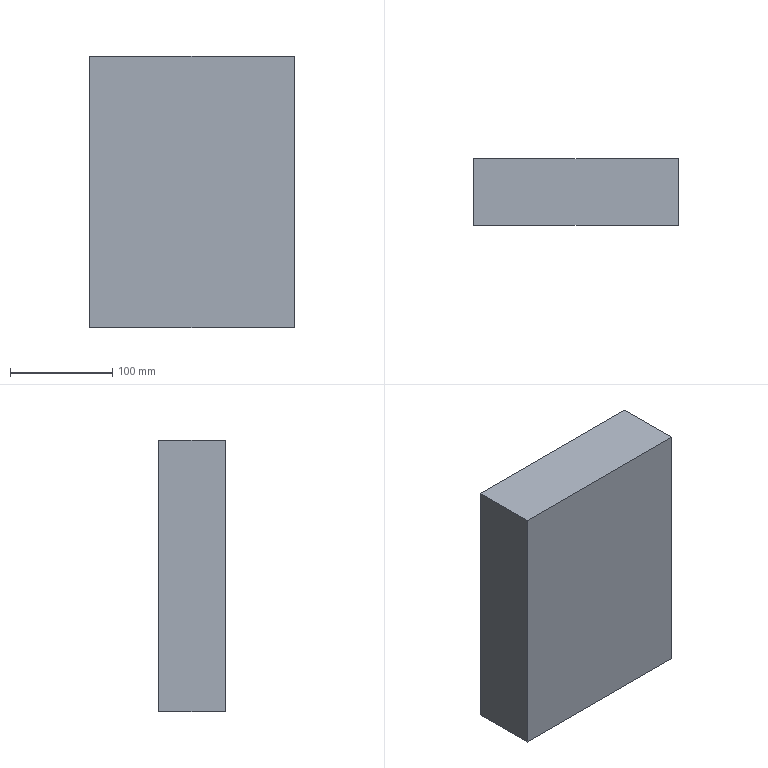Part | STEP file | lll_id3718_x_t | 1 solid | 10 faces | box 200 x 65 x 265 mm | volume 3423738 mm3 | plane 6 | cylinder 2 | cone 2 | commonest cylinder face diameters 17.505 x2
STEP:
#1=CARTESIAN_POINT('',(1843.188,637.5,-370.));
#2=VERTEX_POINT('',#1);
#3=CARTESIAN_POINT('',(1834.435,637.5,-370.));
#4=DIRECTION('',(0.,0.,1.));
#5=DIRECTION('',(1.,0.,0.));
#6=AXIS2_PLACEMENT_3D('',#3,#4,#5);
#7=CIRCLE('',#6,8.752);
#8=EDGE_CURVE('',#2,#2,#7,.T.);
#9=ORIENTED_EDGE('',*,*,#8,.T.);
#10=EDGE_LOOP('',(#9));
#11=FACE_BOUND('',#10,.T.);
#12=CARTESIAN_POINT('',(1809.435,670.,-370.));
#13=VERTEX_POINT('',#12);
#14=CARTESIAN_POINT('',(2009.435,670.,-370.));
#15=VERTEX_POINT('',#14);
#16=CARTESIAN_POINT('',(4038.751,670.,-370.));
#17=DIRECTION('',(1.,0.,0.));
#18=VECTOR('',#17,1.);
#19=LINE('',#16,#18);
#20=EDGE_CURVE('',#13,#15,#19,.T.);
#21=ORIENTED_EDGE('',*,*,#20,.T.);
#22=CARTESIAN_POINT('',(2009.435,605.,-370.));
#23=VERTEX_POINT('',#22);
#24=CARTESIAN_POINT('',(2009.435,1.,-370.));
#25=DIRECTION('',(0.,1.,0.));
#26=VECTOR('',#25,1.);
#27=LINE('',#24,#26);
#28=EDGE_CURVE('',#23,#15,#27,.T.);
#29=ORIENTED_EDGE('',*,*,#28,.F.);
#30=CARTESIAN_POINT('',(1809.435,605.,-370.));
#31=VERTEX_POINT('',#30);
#32=CARTESIAN_POINT('',(4038.751,605.,-370.));
#33=DIRECTION('',(1.,0.,0.));
#34=VECTOR('',#33,1.);
#35=LINE('',#32,#34);
#36=EDGE_CURVE('',#31,#23,#35,.T.);
#37=ORIENTED_EDGE('',*,*,#36,.F.);
#38=CARTESIAN_POINT('',(1809.435,636.5,-370.));
#39=DIRECTION('',(0.,-1.,0.));
#40=VECTOR('',#39,1.);
#41=LINE('',#38,#40);
#42=EDGE_CURVE('',#13,#31,#41,.T.);
#43=ORIENTED_EDGE('',*,*,#42,.F.);
#44=EDGE_LOOP('',(#21,#29,#37,#43));
#45=FACE_BOUND('',#44,.T.);
#46=CARTESIAN_POINT('',(1993.188,637.5,-370.));
#47=VERTEX_POINT('',#46);
#48=CARTESIAN_POINT('',(1984.435,637.5,-370.));
#49=DIRECTION('',(0.,0.,1.));
#50=DIRECTION('',(1.,0.,0.));
#51=AXIS2_PLACEMENT_3D('',#48,#49,#50);
#52=CIRCLE('',#51,8.752);
#53=EDGE_CURVE('',#47,#47,#52,.T.);
#54=ORIENTED_EDGE('',*,*,#53,.T.);
#55=EDGE_LOOP('',(#54));
#56=FACE_BOUND('',#55,.T.);
#57=CARTESIAN_POINT('',(4038.751,1.,-370.));
#58=DIRECTION('',(0.,0.,-1.));
#59=DIRECTION('',(-1.,0.,0.));
#60=AXIS2_PLACEMENT_3D('',#57,#58,#59);
#61=PLANE('',#60);
#62=ADVANCED_FACE('',(#11,#45,#56),#61,.T.);
#63=CARTESIAN_POINT('',(2009.435,605.,-105.));
#64=VERTEX_POINT('',#63);
#65=CARTESIAN_POINT('',(2009.435,605.,-180.));
#66=DIRECTION('',(0.,0.,-1.));
#67=VECTOR('',#66,1.);
#68=LINE('',#65,#67);
#69=EDGE_CURVE('',#64,#23,#68,.T.);
#70=ORIENTED_EDGE('',*,*,#69,.F.);
#71=CARTESIAN_POINT('',(1809.435,605.,-105.));
#72=VERTEX_POINT('',#71);
#73=CARTESIAN_POINT('',(2154.435,605.,-105.));
#74=DIRECTION('',(1.,0.,0.));
#75=VECTOR('',#74,1.);
#76=LINE('',#73,#75);
#77=EDGE_CURVE('',#72,#64,#76,.T.);
#78=ORIENTED_EDGE('',*,*,#77,.F.);
#79=CARTESIAN_POINT('',(1809.435,605.,-180.));
#80=DIRECTION('',(0.,0.,-1.));
#81=VECTOR('',#80,1.);
#82=LINE('',#79,#81);
#83=EDGE_CURVE('',#72,#31,#82,.T.);
#84=ORIENTED_EDGE('',*,*,#83,.T.);
#85=ORIENTED_EDGE('',*,*,#36,.T.);
#86=EDGE_LOOP('',(#70,#78,#84,#85));
#87=FACE_OUTER_BOUND('',#86,.T.);
#88=CARTESIAN_POINT('',(2052.435,605.,-180.));
#89=DIRECTION('',(0.,1.,0.));
#90=DIRECTION('',(1.,0.,0.));
#91=AXIS2_PLACEMENT_3D('',#88,#89,#90);
#92=PLANE('',#91);
#93=ADVANCED_FACE('',(#87),#92,.F.);
#94=ORIENTED_EDGE('',*,*,#83,.F.);
#95=CARTESIAN_POINT('',(1809.435,670.,-105.));
#96=VERTEX_POINT('',#95);
#97=CARTESIAN_POINT('',(1809.435,593.,-105.));
#98=DIRECTION('',(0.,-1.,0.000000092));
#99=VECTOR('',#98,1.);
#100=LINE('',#97,#99);
#101=EDGE_CURVE('',#96,#72,#100,.T.);
#102=ORIENTED_EDGE('',*,*,#101,.F.);
#103=CARTESIAN_POINT('',(1809.435,670.,-180.));
#104=DIRECTION('',(0.,0.,-1.));
#105=VECTOR('',#104,1.);
#106=LINE('',#103,#105);
#107=EDGE_CURVE('',#96,#13,#106,.T.);
#108=ORIENTED_EDGE('',*,*,#107,.T.);
#109=ORIENTED_EDGE('',*,*,#42,.T.);
#110=EDGE_LOOP('',(#94,#102,#108,#109));
#111=FACE_OUTER_BOUND('',#110,.T.);
#112=CARTESIAN_POINT('',(1809.435,636.5,-180.));
#113=DIRECTION('',(1.,0.,0.));
#114=DIRECTION('',(0.,-1.,0.));
#115=AXIS2_PLACEMENT_3D('',#112,#113,#114);
#116=PLANE('',#115);
#117=ADVANCED_FACE('',(#111),#116,.F.);
#118=ORIENTED_EDGE('',*,*,#107,.F.);
#119=CARTESIAN_POINT('',(2009.435,670.,-105.));
#120=VERTEX_POINT('',#119);
#121=CARTESIAN_POINT('',(2154.435,670.,-105.));
#122=DIRECTION('',(1.,0.,0.));
#123=VECTOR('',#122,1.);
#124=LINE('',#121,#123);
#125=EDGE_CURVE('',#96,#120,#124,.T.);
#126=ORIENTED_EDGE('',*,*,#125,.T.);
#127=CARTESIAN_POINT('',(2009.435,670.,-180.));
#128=DIRECTION('',(0.,0.,-1.));
#129=VECTOR('',#128,1.);
#130=LINE('',#127,#129);
#131=EDGE_CURVE('',#120,#15,#130,.T.);
#132=ORIENTED_EDGE('',*,*,#131,.T.);
#133=ORIENTED_EDGE('',*,*,#20,.F.);
#134=EDGE_LOOP('',(#118,#126,#132,#133));
#135=FACE_OUTER_BOUND('',#134,.T.);
#136=CARTESIAN_POINT('',(1983.435,670.,-180.));
#137=DIRECTION('',(0.,1.,0.));
#138=DIRECTION('',(1.,0.,0.));
#139=AXIS2_PLACEMENT_3D('',#136,#137,#138);
#140=PLANE('',#139);
#141=ADVANCED_FACE('',(#135),#140,.T.);
#142=CARTESIAN_POINT('',(2009.435,600.,-105.));
#143=DIRECTION('',(0.,1.,-0.000000092));
#144=VECTOR('',#143,1.);
#145=LINE('',#142,#144);
#146=EDGE_CURVE('',#64,#120,#145,.T.);
#147=ORIENTED_EDGE('',*,*,#146,.F.);
#148=ORIENTED_EDGE('',*,*,#69,.T.);
#149=ORIENTED_EDGE('',*,*,#28,.T.);
#150=ORIENTED_EDGE('',*,*,#131,.F.);
#151=EDGE_LOOP('',(#147,#148,#149,#150));
#152=FACE_OUTER_BOUND('',#151,.T.);
#153=CARTESIAN_POINT('',(2009.435,600.,-180.));
#154=DIRECTION('',(1.,0.,0.));
#155=DIRECTION('',(0.,0.,1.));
#156=AXIS2_PLACEMENT_3D('',#153,#154,#155);
#157=PLANE('',#156);
#158=ADVANCED_FACE('',(#152),#157,.T.);
#159=ORIENTED_EDGE('',*,*,#125,.F.);
#160=ORIENTED_EDGE('',*,*,#101,.T.);
#161=ORIENTED_EDGE('',*,*,#77,.T.);
#162=ORIENTED_EDGE('',*,*,#146,.T.);
#163=EDGE_LOOP('',(#159,#160,#161,#162));
#164=FACE_OUTER_BOUND('',#163,.T.);
#165=CARTESIAN_POINT('',(2154.435,593.,-105.));
#166=DIRECTION('',(0.,-0.000000092,-1.));
#167=DIRECTION('',(-1.,0.,0.));
#168=AXIS2_PLACEMENT_3D('',#165,#166,#167);
#169=PLANE('',#168);
#170=ADVANCED_FACE('',(#164),#169,.F.);
#171=CARTESIAN_POINT('',(1843.188,637.5,-328.747));
#172=VERTEX_POINT('',#171);
#173=CARTESIAN_POINT('',(1834.435,637.5,-328.747));
#174=DIRECTION('',(0.,0.,1.));
#175=DIRECTION('',(1.,0.,0.));
#176=AXIS2_PLACEMENT_3D('',#173,#174,#175);
#177=CIRCLE('',#176,8.752);
#178=EDGE_CURVE('',#172,#172,#177,.T.);
#179=ORIENTED_EDGE('',*,*,#178,.T.);
#180=EDGE_LOOP('',(#179));
#181=FACE_BOUND('',#180,.T.);
#182=ORIENTED_EDGE('',*,*,#8,.F.);
#183=EDGE_LOOP('',(#182));
#184=FACE_BOUND('',#183,.T.);
#185=CARTESIAN_POINT('',(1834.435,637.5,-370.));
#186=DIRECTION('',(0.,0.,1.));
#187=DIRECTION('',(-1.,0.,0.));
#188=AXIS2_PLACEMENT_3D('',#185,#186,#187);
#189=CYLINDRICAL_SURFACE('',#188,8.752);
#190=ADVANCED_FACE('',(#181,#184),#189,.F.);
#191=CARTESIAN_POINT('',(1834.435,637.5,-319.994));
#192=VERTEX_POINT('',#191);
#193=VERTEX_LOOP('',#192);
#194=FACE_BOUND('',#193,.T.);
#195=ORIENTED_EDGE('',*,*,#178,.F.);
#196=EDGE_LOOP('',(#195));
#197=FACE_BOUND('',#196,.T.);
#198=CARTESIAN_POINT('',(1834.435,637.5,-328.747));
#199=DIRECTION('',(0.,0.,-1.));
#200=DIRECTION('',(1.,0.,0.));
#201=AXIS2_PLACEMENT_3D('',#198,#199,#200);
#202=CONICAL_SURFACE('',#201,8.752,45.);
#203=ADVANCED_FACE('',(#194,#197),#202,.F.);
#204=CARTESIAN_POINT('',(1993.188,637.5,-328.747));
#205=VERTEX_POINT('',#204);
#206=CARTESIAN_POINT('',(1984.435,637.5,-328.747));
#207=DIRECTION('',(0.,0.,1.));
#208=DIRECTION('',(1.,0.,0.));
#209=AXIS2_PLACEMENT_3D('',#206,#207,#208);
#210=CIRCLE('',#209,8.752);
#211=EDGE_CURVE('',#205,#205,#210,.T.);
#212=ORIENTED_EDGE('',*,*,#211,.T.);
#213=EDGE_LOOP('',(#212));
#214=FACE_BOUND('',#213,.T.);
#215=ORIENTED_EDGE('',*,*,#53,.F.);
#216=EDGE_LOOP('',(#215));
#217=FACE_BOUND('',#216,.T.);
#218=CARTESIAN_POINT('',(1984.435,637.5,-370.));
#219=DIRECTION('',(0.,0.,1.));
#220=DIRECTION('',(-1.,0.,0.));
#221=AXIS2_PLACEMENT_3D('',#218,#219,#220);
#222=CYLINDRICAL_SURFACE('',#221,8.752);
#223=ADVANCED_FACE('',(#214,#217),#222,.F.);
#224=CARTESIAN_POINT('',(1984.435,637.5,-319.994));
#225=VERTEX_POINT('',#224);
#226=VERTEX_LOOP('',#225);
#227=FACE_BOUND('',#226,.T.);
#228=ORIENTED_EDGE('',*,*,#211,.F.);
#229=EDGE_LOOP('',(#228));
#230=FACE_BOUND('',#229,.T.);
#231=CARTESIAN_POINT('',(1984.435,637.5,-328.747));
#232=DIRECTION('',(0.,0.,-1.));
#233=DIRECTION('',(1.,0.,0.));
#234=AXIS2_PLACEMENT_3D('',#231,#232,#233);
#235=CONICAL_SURFACE('',#234,8.752,45.);
#236=ADVANCED_FACE('',(#227,#230),#235,.F.);
#237=CLOSED_SHELL('',(#62,#93,#117,#141,#158,#170,#190,#203,#223,#236));
#238=MANIFOLD_SOLID_BREP('',#237);
#239=(LENGTH_UNIT()NAMED_UNIT(*)SI_UNIT(.MILLI.,.METRE.));
#240=UNCERTAINTY_MEASURE_WITH_UNIT(LENGTH_MEASURE(0.00002),#239,'','');
#241=(NAMED_UNIT(*)PLANE_ANGLE_UNIT()SI_UNIT($,.RADIAN.));
#242=PLANE_ANGLE_MEASURE_WITH_UNIT(PLANE_ANGLE_MEASURE(0.01745),#241);
#243=DIMENSIONAL_EXPONENTS(0.,0.,0.,0.,0.,0.,0.);
#244=(CONVERSION_BASED_UNIT('DEGREE',#242)NAMED_UNIT(#243)PLANE_ANGLE_UNIT());
#245=(NAMED_UNIT(*)SI_UNIT($,.STERADIAN.)SOLID_ANGLE_UNIT());
#246=(GEOMETRIC_REPRESENTATION_CONTEXT(3)GLOBAL_UNCERTAINTY_ASSIGNED_CONTEXT((#240))GLOBAL_UNIT_ASSIGNED_CONTEXT((#239,#244,#245))REPRESENTATION_CONTEXT('',''));
#247=ADVANCED_BREP_SHAPE_REPRESENTATION('',(#238),#246);